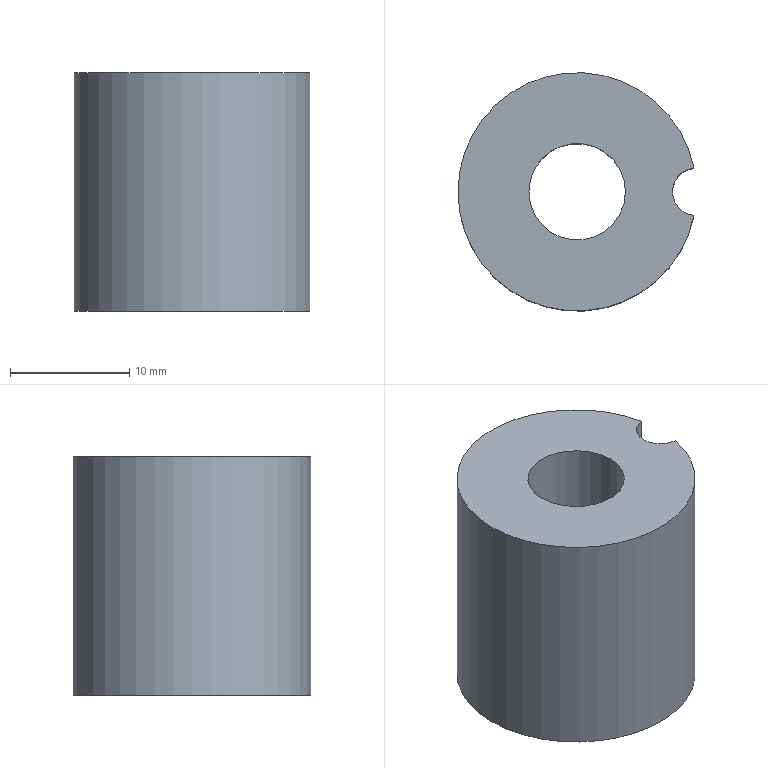Part | NX | features solid 2 | 1 solid | 7 faces | box 19.8 x 20 x 20 mm | volume 4254 mm3 | cylinder 4 | plane 3 | commonest cylinder face diameters 4 x1 8.1 x1 12.6 x1 20 x1
STEP:
#1=CARTESIAN_POINT('',(-811.207,-376.305,38.));
#2=VERTEX_POINT('',#1);
#3=CARTESIAN_POINT('',(-811.207,-376.305,58.));
#4=VERTEX_POINT('',#3);
#5=CARTESIAN_POINT('',(-811.207,-376.305,48.));
#6=DIRECTION('',(0.,0.,1.));
#7=VECTOR('',#6,1000.);
#8=LINE('',#5,#7);
#9=EDGE_CURVE('',#2,#4,#8,.T.);
#10=ORIENTED_EDGE('',*,*,#9,.F.);
#11=CARTESIAN_POINT('',(-811.207,-380.285,38.));
#12=VERTEX_POINT('',#11);
#13=CARTESIAN_POINT('',(-821.007,-378.295,38.));
#14=DIRECTION('',(0.,0.,1.));
#15=DIRECTION('',(1.,0.,0.));
#16=AXIS2_PLACEMENT_3D('',#13,#14,#15);
#17=CIRCLE('',#16,10.);
#18=EDGE_CURVE('',#2,#12,#17,.T.);
#19=ORIENTED_EDGE('',*,*,#18,.T.);
#20=CARTESIAN_POINT('',(-811.207,-380.285,58.));
#21=VERTEX_POINT('',#20);
#22=CARTESIAN_POINT('',(-811.207,-380.285,48.));
#23=DIRECTION('',(0.,0.,1.));
#24=VECTOR('',#23,1000.);
#25=LINE('',#22,#24);
#26=EDGE_CURVE('',#21,#12,#25,.F.);
#27=ORIENTED_EDGE('',*,*,#26,.F.);
#28=CARTESIAN_POINT('',(-821.007,-378.295,58.));
#29=DIRECTION('',(0.,0.,1.));
#30=DIRECTION('',(1.,0.,0.));
#31=AXIS2_PLACEMENT_3D('',#28,#29,#30);
#32=CIRCLE('',#31,10.);
#33=EDGE_CURVE('',#4,#21,#32,.T.);
#34=ORIENTED_EDGE('',*,*,#33,.F.);
#35=EDGE_LOOP('',(#10,#19,#27,#34));
#36=FACE_BOUND('',#35,.T.);
#37=CARTESIAN_POINT('',(-821.007,-378.295,38.));
#38=DIRECTION('',(0.,0.,1.));
#39=DIRECTION('',(1.,0.,0.));
#40=AXIS2_PLACEMENT_3D('',#37,#38,#39);
#41=CYLINDRICAL_SURFACE('',#40,10.);
#42=ADVANCED_FACE('',(#36),#41,.T.);
#43=CARTESIAN_POINT('',(-814.707,-378.295,38.));
#44=VERTEX_POINT('',#43);
#45=CARTESIAN_POINT('',(-821.007,-378.295,38.));
#46=DIRECTION('',(0.,0.,1.));
#47=DIRECTION('',(1.,0.,0.));
#48=AXIS2_PLACEMENT_3D('',#45,#46,#47);
#49=CIRCLE('',#48,6.3);
#50=EDGE_CURVE('',#44,#44,#49,.T.);
#51=ORIENTED_EDGE('',*,*,#50,.T.);
#52=EDGE_LOOP('',(#51));
#53=FACE_BOUND('',#52,.T.);
#54=ORIENTED_EDGE('',*,*,#18,.F.);
#55=CARTESIAN_POINT('',(-811.007,-378.295,38.));
#56=DIRECTION('',(0.,0.,1.));
#57=DIRECTION('',(1.,0.,0.));
#58=AXIS2_PLACEMENT_3D('',#55,#56,#57);
#59=CIRCLE('',#58,2.);
#60=EDGE_CURVE('',#2,#12,#59,.T.);
#61=ORIENTED_EDGE('',*,*,#60,.T.);
#62=EDGE_LOOP('',(#54,#61));
#63=FACE_BOUND('',#62,.T.);
#64=CARTESIAN_POINT('',(-821.007,-378.295,38.));
#65=DIRECTION('',(0.,0.,1.));
#66=DIRECTION('',(1.,0.,0.));
#67=AXIS2_PLACEMENT_3D('',#64,#65,#66);
#68=PLANE('',#67);
#69=ADVANCED_FACE('',(#53,#63),#68,.F.);
#70=CARTESIAN_POINT('',(-816.957,-378.295,58.));
#71=VERTEX_POINT('',#70);
#72=CARTESIAN_POINT('',(-821.007,-378.295,58.));
#73=DIRECTION('',(0.,0.,1.));
#74=DIRECTION('',(1.,0.,0.));
#75=AXIS2_PLACEMENT_3D('',#72,#73,#74);
#76=CIRCLE('',#75,4.05);
#77=EDGE_CURVE('',#71,#71,#76,.T.);
#78=ORIENTED_EDGE('',*,*,#77,.F.);
#79=EDGE_LOOP('',(#78));
#80=FACE_BOUND('',#79,.T.);
#81=CARTESIAN_POINT('',(-811.007,-378.295,58.));
#82=DIRECTION('',(0.,0.,1.));
#83=DIRECTION('',(1.,0.,0.));
#84=AXIS2_PLACEMENT_3D('',#81,#82,#83);
#85=CIRCLE('',#84,2.);
#86=EDGE_CURVE('',#4,#21,#85,.T.);
#87=ORIENTED_EDGE('',*,*,#86,.F.);
#88=ORIENTED_EDGE('',*,*,#33,.T.);
#89=EDGE_LOOP('',(#87,#88));
#90=FACE_BOUND('',#89,.T.);
#91=CARTESIAN_POINT('',(-821.007,-378.295,58.));
#92=DIRECTION('',(0.,0.,1.));
#93=DIRECTION('',(1.,0.,0.));
#94=AXIS2_PLACEMENT_3D('',#91,#92,#93);
#95=PLANE('',#94);
#96=ADVANCED_FACE('',(#80,#90),#95,.T.);
#97=ORIENTED_EDGE('',*,*,#50,.F.);
#98=EDGE_LOOP('',(#97));
#99=FACE_BOUND('',#98,.T.);
#100=CARTESIAN_POINT('',(-814.707,-378.295,50.));
#101=VERTEX_POINT('',#100);
#102=CARTESIAN_POINT('',(-821.007,-378.295,50.));
#103=DIRECTION('',(0.,0.,1.));
#104=DIRECTION('',(1.,0.,0.));
#105=AXIS2_PLACEMENT_3D('',#102,#103,#104);
#106=CIRCLE('',#105,6.3);
#107=EDGE_CURVE('',#101,#101,#106,.T.);
#108=ORIENTED_EDGE('',*,*,#107,.T.);
#109=EDGE_LOOP('',(#108));
#110=FACE_BOUND('',#109,.T.);
#111=CARTESIAN_POINT('',(-821.007,-378.295,38.));
#112=DIRECTION('',(0.,0.,1.));
#113=DIRECTION('',(1.,0.,0.));
#114=AXIS2_PLACEMENT_3D('',#111,#112,#113);
#115=CYLINDRICAL_SURFACE('',#114,6.3);
#116=ADVANCED_FACE('',(#99,#110),#115,.F.);
#117=CARTESIAN_POINT('',(-816.957,-378.295,50.));
#118=VERTEX_POINT('',#117);
#119=CARTESIAN_POINT('',(-821.007,-378.295,50.));
#120=DIRECTION('',(0.,0.,1.));
#121=DIRECTION('',(1.,0.,0.));
#122=AXIS2_PLACEMENT_3D('',#119,#120,#121);
#123=CIRCLE('',#122,4.05);
#124=EDGE_CURVE('',#118,#118,#123,.T.);
#125=ORIENTED_EDGE('',*,*,#124,.T.);
#126=EDGE_LOOP('',(#125));
#127=FACE_BOUND('',#126,.T.);
#128=ORIENTED_EDGE('',*,*,#107,.F.);
#129=EDGE_LOOP('',(#128));
#130=FACE_BOUND('',#129,.T.);
#131=CARTESIAN_POINT('',(-821.007,-378.295,50.));
#132=DIRECTION('',(0.,0.,1.));
#133=DIRECTION('',(1.,0.,0.));
#134=AXIS2_PLACEMENT_3D('',#131,#132,#133);
#135=PLANE('',#134);
#136=ADVANCED_FACE('',(#127,#130),#135,.F.);
#137=ORIENTED_EDGE('',*,*,#9,.T.);
#138=ORIENTED_EDGE('',*,*,#86,.T.);
#139=ORIENTED_EDGE('',*,*,#26,.T.);
#140=ORIENTED_EDGE('',*,*,#60,.F.);
#141=EDGE_LOOP('',(#137,#138,#139,#140));
#142=FACE_BOUND('',#141,.T.);
#143=CARTESIAN_POINT('',(-811.007,-378.295,38.));
#144=DIRECTION('',(0.,0.,1.));
#145=DIRECTION('',(1.,0.,0.));
#146=AXIS2_PLACEMENT_3D('',#143,#144,#145);
#147=CYLINDRICAL_SURFACE('',#146,2.);
#148=ADVANCED_FACE('',(#142),#147,.F.);
#149=ORIENTED_EDGE('',*,*,#77,.T.);
#150=EDGE_LOOP('',(#149));
#151=FACE_BOUND('',#150,.T.);
#152=ORIENTED_EDGE('',*,*,#124,.F.);
#153=EDGE_LOOP('',(#152));
#154=FACE_BOUND('',#153,.T.);
#155=CARTESIAN_POINT('',(-821.007,-378.295,38.));
#156=DIRECTION('',(0.,0.,1.));
#157=DIRECTION('',(1.,0.,0.));
#158=AXIS2_PLACEMENT_3D('',#155,#156,#157);
#159=CYLINDRICAL_SURFACE('',#158,4.05);
#160=ADVANCED_FACE('',(#151,#154),#159,.F.);
#161=CLOSED_SHELL('',(#42,#69,#96,#116,#136,#148,#160));
#162=MANIFOLD_SOLID_BREP('',#161);
#163=(LENGTH_UNIT()NAMED_UNIT(*)SI_UNIT(.MILLI.,.METRE.));
#164=UNCERTAINTY_MEASURE_WITH_UNIT(LENGTH_MEASURE(0.00001),#163,'','');
#165=(NAMED_UNIT(*)PLANE_ANGLE_UNIT()SI_UNIT($,.RADIAN.));
#166=(NAMED_UNIT(*)SI_UNIT($,.STERADIAN.)SOLID_ANGLE_UNIT());
#167=(GEOMETRIC_REPRESENTATION_CONTEXT(3)GLOBAL_UNCERTAINTY_ASSIGNED_CONTEXT((#164))GLOBAL_UNIT_ASSIGNED_CONTEXT((#163,#165,#166))REPRESENTATION_CONTEXT('',''));
#168=ADVANCED_BREP_SHAPE_REPRESENTATION('',(#162),#167);